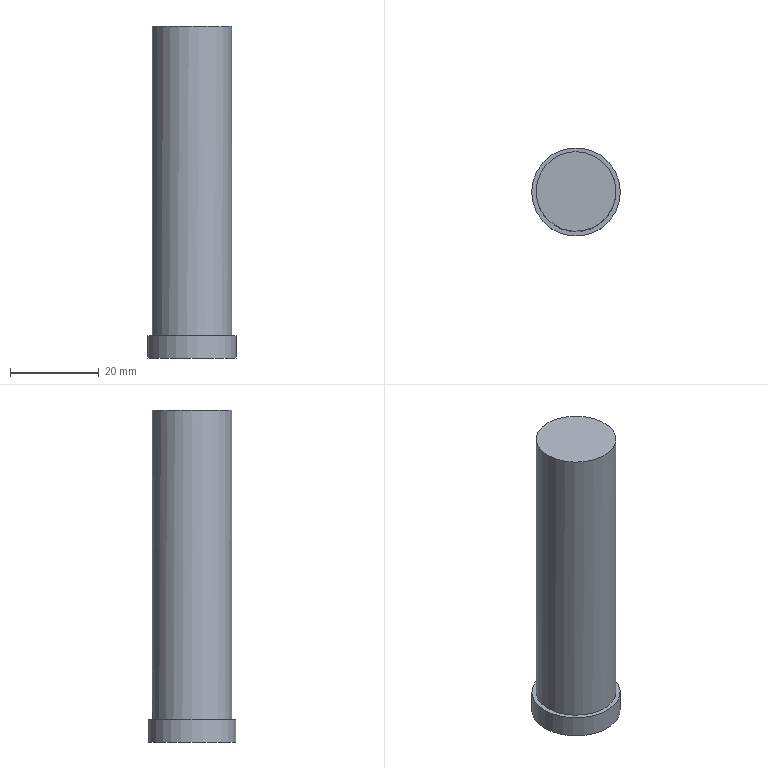Part | NX | features 23 2 | 1 solid | 5 faces | box 20 x 20 x 75 mm | volume 19384 mm3 | plane 3 | cylinder 2 | commonest cylinder face diameters 18 x1 20 x1
STEP:
#1=CARTESIAN_POINT('',(3252.,124.,-18.));
#2=VERTEX_POINT('',#1);
#3=CARTESIAN_POINT('',(3252.,115.,-18.));
#4=DIRECTION('',(0.,0.000000004,1.));
#5=DIRECTION('',(0.,1.,-0.000000004));
#6=AXIS2_PLACEMENT_3D('',#3,#4,#5);
#7=CIRCLE('',#6,9.);
#8=EDGE_CURVE('',#2,#2,#7,.T.);
#9=ORIENTED_EDGE('',*,*,#8,.F.);
#10=EDGE_LOOP('',(#9));
#11=FACE_BOUND('',#10,.T.);
#12=CARTESIAN_POINT('',(3243.,115.,-88.));
#13=VERTEX_POINT('',#12);
#14=CARTESIAN_POINT('',(3252.,115.,-88.));
#15=DIRECTION('',(0.,0.,1.));
#16=DIRECTION('',(-1.,0.,0.));
#17=AXIS2_PLACEMENT_3D('',#14,#15,#16);
#18=CIRCLE('',#17,9.);
#19=EDGE_CURVE('',#13,#13,#18,.T.);
#20=ORIENTED_EDGE('',*,*,#19,.T.);
#21=EDGE_LOOP('',(#20));
#22=FACE_BOUND('',#21,.T.);
#23=CARTESIAN_POINT('',(3252.,115.,-399.));
#24=DIRECTION('',(0.,0.,1.));
#25=DIRECTION('',(-1.,0.,0.));
#26=AXIS2_PLACEMENT_3D('',#23,#24,#25);
#27=CYLINDRICAL_SURFACE('',#26,9.);
#28=ADVANCED_FACE('',(#11,#22),#27,.T.);
#29=ORIENTED_EDGE('',*,*,#8,.T.);
#30=EDGE_LOOP('',(#29));
#31=FACE_BOUND('',#30,.T.);
#32=CARTESIAN_POINT('',(3188.159,111.584,-18.));
#33=DIRECTION('',(0.,0.000000004,1.));
#34=DIRECTION('',(-0.9367,0.3502,-0.000000001));
#35=AXIS2_PLACEMENT_3D('',#32,#33,#34);
#36=PLANE('',#35);
#37=ADVANCED_FACE('',(#31),#36,.T.);
#38=CARTESIAN_POINT('',(3242.,115.,-88.));
#39=VERTEX_POINT('',#38);
#40=CARTESIAN_POINT('',(3252.,115.,-88.));
#41=DIRECTION('',(0.,0.,-1.));
#42=DIRECTION('',(-1.,0.,0.));
#43=AXIS2_PLACEMENT_3D('',#40,#41,#42);
#44=CIRCLE('',#43,10.);
#45=EDGE_CURVE('',#39,#39,#44,.T.);
#46=ORIENTED_EDGE('',*,*,#45,.F.);
#47=EDGE_LOOP('',(#46));
#48=FACE_BOUND('',#47,.T.);
#49=ORIENTED_EDGE('',*,*,#19,.F.);
#50=EDGE_LOOP('',(#49));
#51=FACE_BOUND('',#50,.T.);
#52=CARTESIAN_POINT('',(3252.,115.,-88.));
#53=DIRECTION('',(0.,0.,-1.));
#54=DIRECTION('',(1.,0.,0.));
#55=AXIS2_PLACEMENT_3D('',#52,#53,#54);
#56=PLANE('',#55);
#57=ADVANCED_FACE('',(#48,#51),#56,.F.);
#58=CARTESIAN_POINT('',(3242.,115.,-93.));
#59=VERTEX_POINT('',#58);
#60=CARTESIAN_POINT('',(3252.,115.,-93.));
#61=DIRECTION('',(0.,0.,1.));
#62=DIRECTION('',(-1.,0.,0.));
#63=AXIS2_PLACEMENT_3D('',#60,#61,#62);
#64=CIRCLE('',#63,10.);
#65=EDGE_CURVE('',#59,#59,#64,.T.);
#66=ORIENTED_EDGE('',*,*,#65,.F.);
#67=EDGE_LOOP('',(#66));
#68=FACE_BOUND('',#67,.T.);
#69=CARTESIAN_POINT('',(1598.5,-193.,-93.));
#70=DIRECTION('',(0.,0.,-1.));
#71=DIRECTION('',(-1.,0.,0.));
#72=AXIS2_PLACEMENT_3D('',#69,#70,#71);
#73=PLANE('',#72);
#74=ADVANCED_FACE('',(#68),#73,.T.);
#75=ORIENTED_EDGE('',*,*,#45,.T.);
#76=EDGE_LOOP('',(#75));
#77=FACE_BOUND('',#76,.T.);
#78=ORIENTED_EDGE('',*,*,#65,.T.);
#79=EDGE_LOOP('',(#78));
#80=FACE_BOUND('',#79,.T.);
#81=CARTESIAN_POINT('',(3252.,115.,-399.));
#82=DIRECTION('',(0.,0.,1.));
#83=DIRECTION('',(-1.,0.,0.));
#84=AXIS2_PLACEMENT_3D('',#81,#82,#83);
#85=CYLINDRICAL_SURFACE('',#84,10.);
#86=ADVANCED_FACE('',(#77,#80),#85,.T.);
#87=CLOSED_SHELL('',(#28,#37,#57,#74,#86));
#88=MANIFOLD_SOLID_BREP('',#87);
#89=(LENGTH_UNIT()NAMED_UNIT(*)SI_UNIT(.MILLI.,.METRE.));
#90=UNCERTAINTY_MEASURE_WITH_UNIT(LENGTH_MEASURE(0.00001),#89,'','');
#91=(NAMED_UNIT(*)PLANE_ANGLE_UNIT()SI_UNIT($,.RADIAN.));
#92=(NAMED_UNIT(*)SI_UNIT($,.STERADIAN.)SOLID_ANGLE_UNIT());
#93=(GEOMETRIC_REPRESENTATION_CONTEXT(3)GLOBAL_UNCERTAINTY_ASSIGNED_CONTEXT((#90))GLOBAL_UNIT_ASSIGNED_CONTEXT((#89,#91,#92))REPRESENTATION_CONTEXT('',''));
#94=ADVANCED_BREP_SHAPE_REPRESENTATION('',(#88),#93);